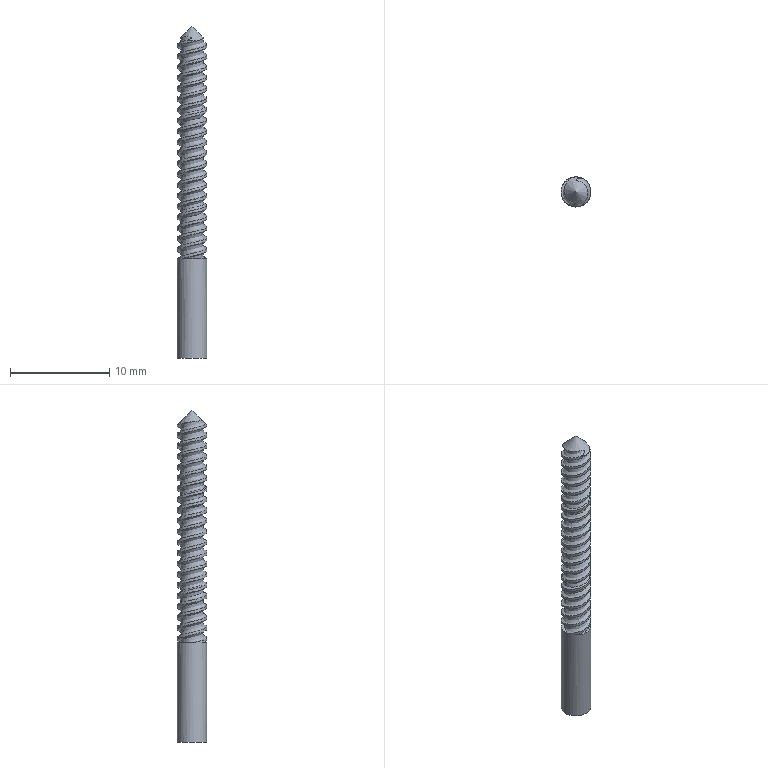Part | NX | features BREP 1, DATUM_CSYS 1 | 1 solid | 32 faces | box 3 x 3.001 x 33.5 mm | volume 185.13 mm3 | cylinder 22 | spline 6 | plane 3 | cone 1 | commonest cylinder face diameters 3 x22